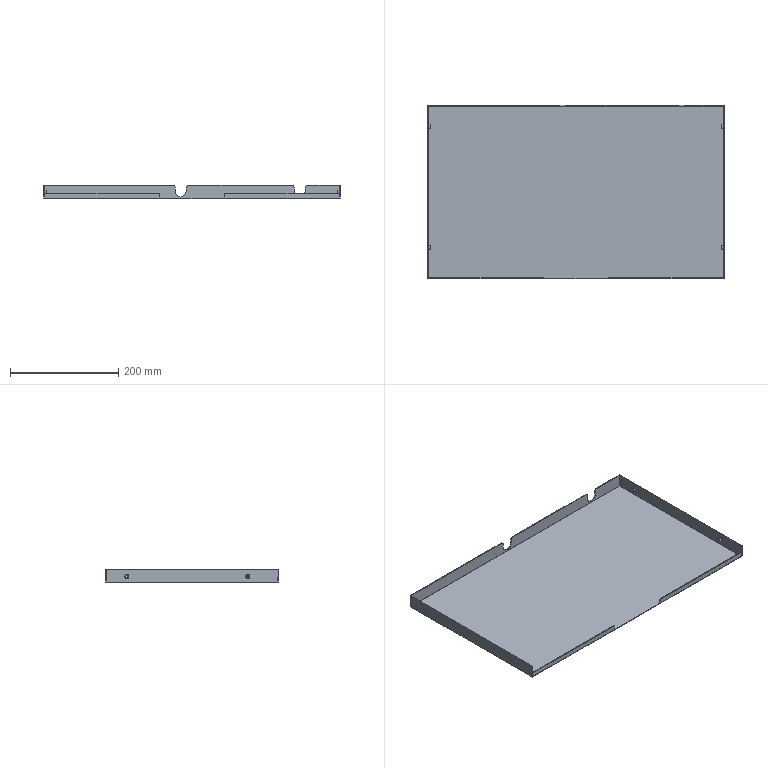Part | STEP file | FHD-021-007-B TZD10S drawer 2 | 1 solid | 76 faces | box 548 x 320 x 25 mm | volume 247788 mm3 | plane 48 | cylinder 24 | spline 4 | commonest cylinder face diameters 0.4 x5 2.8 x5 3.3 x4 8.1 x4 10 x4 20 x2